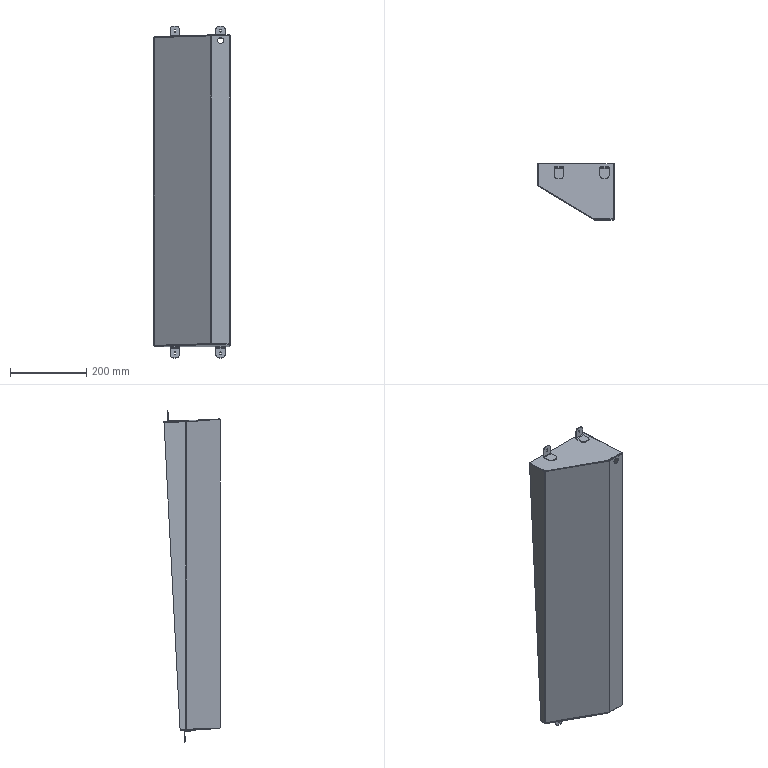Part | STEP file | Sink bevel V1.201001 | 5 solids | 126 faces | box 200 x 147.478 x 872.907 mm | volume 358159 mm3 | plane 72 | cylinder 48 | spline 6 | commonest cylinder face diameters 20 x16 3.5 x12 3 x5 5 x5 4 x4 8 x4